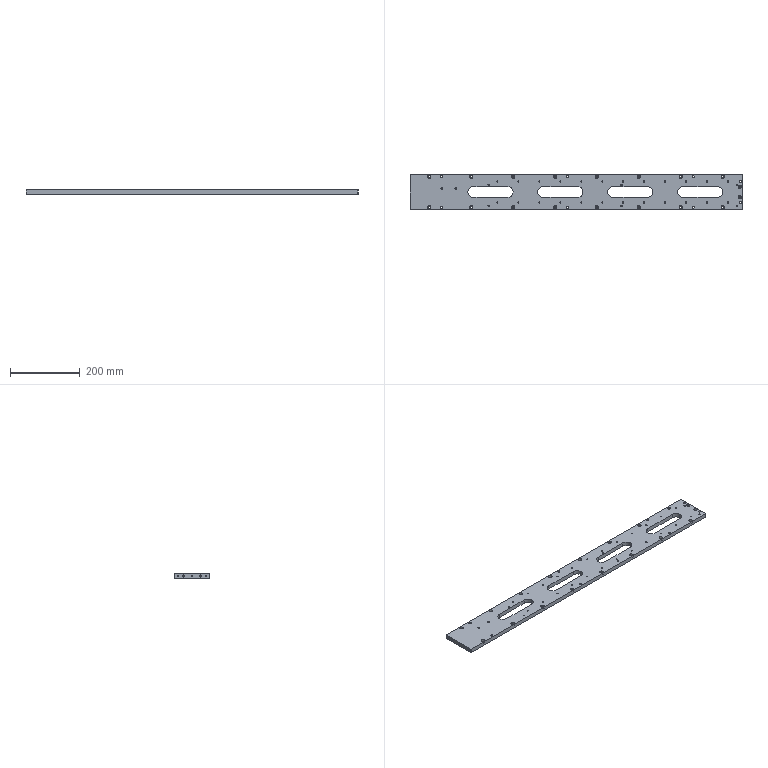Part | SolidWorks | features HoleWzd 9, LPattern 3, Chamfer 1, Extrusion 1, ICE 1 | 1 solid | 220 faces | box 950 x 100 x 12 mm | volume 942474 mm3 | cylinder 174 | plane 36 | cone 10 | commonest cylinder face diameters 3.3 x48 5.5 x36 10 x36 6 x20 4 x12 30 x12